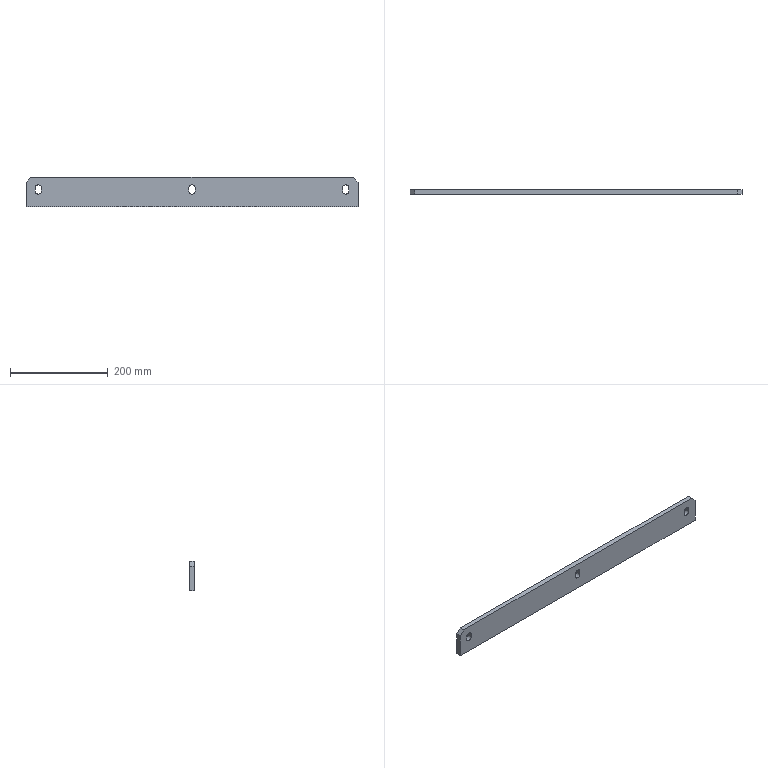Part | NX | features solid 2 | 1 solid | 20 faces | box 680 x 10 x 60 mm | volume 400678 mm3 | plane 14 | cylinder 6 | commonest cylinder face diameters 13 x6
STEP:
#1=CARTESIAN_POINT('',(-390.,10.,-530.));
#2=VERTEX_POINT('',#1);
#3=CARTESIAN_POINT('',(-380.,10.,-540.));
#4=VERTEX_POINT('',#3);
#5=CARTESIAN_POINT('',(-380.,10.,-540.));
#6=DIRECTION('',(0.7071,0.,-0.7071));
#7=VECTOR('',#6,1000.);
#8=LINE('',#5,#7);
#9=EDGE_CURVE('',#2,#4,#8,.T.);
#10=ORIENTED_EDGE('',*,*,#9,.F.);
#11=CARTESIAN_POINT('',(-390.,0.,-530.));
#12=VERTEX_POINT('',#11);
#13=CARTESIAN_POINT('',(-390.,0.,-530.));
#14=DIRECTION('',(0.,1.,0.));
#15=VECTOR('',#14,1000.);
#16=LINE('',#13,#15);
#17=EDGE_CURVE('',#12,#2,#16,.T.);
#18=ORIENTED_EDGE('',*,*,#17,.F.);
#19=CARTESIAN_POINT('',(-380.,0.,-540.));
#20=VERTEX_POINT('',#19);
#21=CARTESIAN_POINT('',(-655.,0.,-265.));
#22=DIRECTION('',(-0.7071,0.,0.7071));
#23=VECTOR('',#22,1000.);
#24=LINE('',#21,#23);
#25=EDGE_CURVE('',#20,#12,#24,.T.);
#26=ORIENTED_EDGE('',*,*,#25,.F.);
#27=CARTESIAN_POINT('',(-380.,10.,-540.));
#28=DIRECTION('',(0.,-1.,0.));
#29=VECTOR('',#28,1000.);
#30=LINE('',#27,#29);
#31=EDGE_CURVE('',#4,#20,#30,.T.);
#32=ORIENTED_EDGE('',*,*,#31,.F.);
#33=EDGE_LOOP('',(#10,#18,#26,#32));
#34=FACE_BOUND('',#33,.T.);
#35=CARTESIAN_POINT('',(-380.,10.,-540.));
#36=DIRECTION('',(-0.7071,0.,-0.7071));
#37=DIRECTION('',(-0.7071,0.,0.7071));
#38=AXIS2_PLACEMENT_3D('',#35,#36,#37);
#39=PLANE('',#38);
#40=ADVANCED_FACE('',(#34),#39,.F.);
#41=CARTESIAN_POINT('',(-1060.,10.,-540.));
#42=VERTEX_POINT('',#41);
#43=CARTESIAN_POINT('',(-1050.,10.,-530.));
#44=VERTEX_POINT('',#43);
#45=CARTESIAN_POINT('',(-1050.,10.,-530.));
#46=DIRECTION('',(0.7071,0.,0.7071));
#47=VECTOR('',#46,1000.);
#48=LINE('',#45,#47);
#49=EDGE_CURVE('',#42,#44,#48,.T.);
#50=ORIENTED_EDGE('',*,*,#49,.F.);
#51=CARTESIAN_POINT('',(-1060.,0.,-540.));
#52=VERTEX_POINT('',#51);
#53=CARTESIAN_POINT('',(-1060.,10.,-540.));
#54=DIRECTION('',(0.,1.,0.));
#55=VECTOR('',#54,1000.);
#56=LINE('',#53,#55);
#57=EDGE_CURVE('',#52,#42,#56,.T.);
#58=ORIENTED_EDGE('',*,*,#57,.F.);
#59=CARTESIAN_POINT('',(-1050.,0.,-530.));
#60=VERTEX_POINT('',#59);
#61=CARTESIAN_POINT('',(-1055.,0.,-535.));
#62=DIRECTION('',(-0.7071,0.,-0.7071));
#63=VECTOR('',#62,1000.);
#64=LINE('',#61,#63);
#65=EDGE_CURVE('',#60,#52,#64,.T.);
#66=ORIENTED_EDGE('',*,*,#65,.F.);
#67=CARTESIAN_POINT('',(-1050.,0.,-530.));
#68=DIRECTION('',(0.,-1.,0.));
#69=VECTOR('',#68,1000.);
#70=LINE('',#67,#69);
#71=EDGE_CURVE('',#44,#60,#70,.T.);
#72=ORIENTED_EDGE('',*,*,#71,.F.);
#73=EDGE_LOOP('',(#50,#58,#66,#72));
#74=FACE_BOUND('',#73,.T.);
#75=CARTESIAN_POINT('',(-1050.,0.,-530.));
#76=DIRECTION('',(0.7071,0.,-0.7071));
#77=DIRECTION('',(0.,-1.,0.));
#78=AXIS2_PLACEMENT_3D('',#75,#76,#77);
#79=PLANE('',#78);
#80=ADVANCED_FACE('',(#74),#79,.F.);
#81=CARTESIAN_POINT('',(-1028.5,0.,-558.001));
#82=VERTEX_POINT('',#81);
#83=CARTESIAN_POINT('',(-1028.5,0.,-552.001));
#84=VERTEX_POINT('',#83);
#85=CARTESIAN_POINT('',(-1028.5,0.,-600.));
#86=DIRECTION('',(0.,0.,1.));
#87=VECTOR('',#86,1000.);
#88=LINE('',#85,#87);
#89=EDGE_CURVE('',#82,#84,#88,.T.);
#90=ORIENTED_EDGE('',*,*,#89,.T.);
#91=CARTESIAN_POINT('',(-1028.5,10.,-552.001));
#92=VERTEX_POINT('',#91);
#93=CARTESIAN_POINT('',(-1028.5,-672.715,-552.001));
#94=DIRECTION('',(0.,1.,0.));
#95=VECTOR('',#94,1000.);
#96=LINE('',#93,#95);
#97=EDGE_CURVE('',#84,#92,#96,.T.);
#98=ORIENTED_EDGE('',*,*,#97,.T.);
#99=CARTESIAN_POINT('',(-1028.5,10.,-558.001));
#100=VERTEX_POINT('',#99);
#101=CARTESIAN_POINT('',(-1028.5,10.,-552.001));
#102=DIRECTION('',(0.,0.,-1.));
#103=VECTOR('',#102,1000.);
#104=LINE('',#101,#103);
#105=EDGE_CURVE('',#92,#100,#104,.T.);
#106=ORIENTED_EDGE('',*,*,#105,.T.);
#107=CARTESIAN_POINT('',(-1028.5,-672.715,-558.001));
#108=DIRECTION('',(0.,1.,0.));
#109=VECTOR('',#108,1000.);
#110=LINE('',#107,#109);
#111=EDGE_CURVE('',#82,#100,#110,.T.);
#112=ORIENTED_EDGE('',*,*,#111,.F.);
#113=EDGE_LOOP('',(#90,#98,#106,#112));
#114=FACE_BOUND('',#113,.T.);
#115=CARTESIAN_POINT('',(-1028.5,-672.715,-552.001));
#116=DIRECTION('',(1.,0.,0.));
#117=DIRECTION('',(0.,0.,-1.));
#118=AXIS2_PLACEMENT_3D('',#115,#116,#117);
#119=PLANE('',#118);
#120=ADVANCED_FACE('',(#114),#119,.F.);
#121=CARTESIAN_POINT('',(-1041.5,0.,-552.001));
#122=VERTEX_POINT('',#121);
#123=CARTESIAN_POINT('',(-1035.,0.,-552.001));
#124=DIRECTION('',(0.,-1.,0.));
#125=DIRECTION('',(1.,0.,0.));
#126=AXIS2_PLACEMENT_3D('',#123,#124,#125);
#127=CIRCLE('',#126,6.5);
#128=EDGE_CURVE('',#84,#122,#127,.T.);
#129=ORIENTED_EDGE('',*,*,#128,.T.);
#130=CARTESIAN_POINT('',(-1041.5,10.,-552.001));
#131=VERTEX_POINT('',#130);
#132=CARTESIAN_POINT('',(-1041.5,-672.715,-552.001));
#133=DIRECTION('',(0.,1.,0.));
#134=VECTOR('',#133,1000.);
#135=LINE('',#132,#134);
#136=EDGE_CURVE('',#122,#131,#135,.T.);
#137=ORIENTED_EDGE('',*,*,#136,.T.);
#138=CARTESIAN_POINT('',(-1035.,10.,-552.001));
#139=DIRECTION('',(0.,1.,0.));
#140=DIRECTION('',(-1.,0.,0.));
#141=AXIS2_PLACEMENT_3D('',#138,#139,#140);
#142=CIRCLE('',#141,6.5);
#143=EDGE_CURVE('',#131,#92,#142,.T.);
#144=ORIENTED_EDGE('',*,*,#143,.T.);
#145=ORIENTED_EDGE('',*,*,#97,.F.);
#146=EDGE_LOOP('',(#129,#137,#144,#145));
#147=FACE_BOUND('',#146,.T.);
#148=CARTESIAN_POINT('',(-1035.,-672.715,-552.001));
#149=DIRECTION('',(0.,1.,0.));
#150=DIRECTION('',(-1.,0.,0.));
#151=AXIS2_PLACEMENT_3D('',#148,#149,#150);
#152=CYLINDRICAL_SURFACE('',#151,6.5);
#153=ADVANCED_FACE('',(#147),#152,.F.);
#154=CARTESIAN_POINT('',(-1041.5,0.,-558.001));
#155=VERTEX_POINT('',#154);
#156=CARTESIAN_POINT('',(-1041.5,0.,-600.));
#157=DIRECTION('',(0.,0.,-1.));
#158=VECTOR('',#157,1000.);
#159=LINE('',#156,#158);
#160=EDGE_CURVE('',#122,#155,#159,.T.);
#161=ORIENTED_EDGE('',*,*,#160,.T.);
#162=CARTESIAN_POINT('',(-1041.5,10.,-558.001));
#163=VERTEX_POINT('',#162);
#164=CARTESIAN_POINT('',(-1041.5,-672.715,-558.001));
#165=DIRECTION('',(0.,1.,0.));
#166=VECTOR('',#165,1000.);
#167=LINE('',#164,#166);
#168=EDGE_CURVE('',#155,#163,#167,.T.);
#169=ORIENTED_EDGE('',*,*,#168,.T.);
#170=CARTESIAN_POINT('',(-1041.5,10.,-552.001));
#171=DIRECTION('',(0.,0.,1.));
#172=VECTOR('',#171,1000.);
#173=LINE('',#170,#172);
#174=EDGE_CURVE('',#163,#131,#173,.T.);
#175=ORIENTED_EDGE('',*,*,#174,.T.);
#176=ORIENTED_EDGE('',*,*,#136,.F.);
#177=EDGE_LOOP('',(#161,#169,#175,#176));
#178=FACE_BOUND('',#177,.T.);
#179=CARTESIAN_POINT('',(-1041.5,-672.715,-552.001));
#180=DIRECTION('',(-1.,0.,0.));
#181=DIRECTION('',(0.,1.,0.));
#182=AXIS2_PLACEMENT_3D('',#179,#180,#181);
#183=PLANE('',#182);
#184=ADVANCED_FACE('',(#178),#183,.F.);
#185=CARTESIAN_POINT('',(-1035.,0.,-558.001));
#186=DIRECTION('',(0.,-1.,0.));
#187=DIRECTION('',(1.,0.,0.));
#188=AXIS2_PLACEMENT_3D('',#185,#186,#187);
#189=CIRCLE('',#188,6.5);
#190=EDGE_CURVE('',#155,#82,#189,.T.);
#191=ORIENTED_EDGE('',*,*,#190,.T.);
#192=ORIENTED_EDGE('',*,*,#111,.T.);
#193=CARTESIAN_POINT('',(-1035.,10.,-558.001));
#194=DIRECTION('',(0.,1.,0.));
#195=DIRECTION('',(1.,0.,0.));
#196=AXIS2_PLACEMENT_3D('',#193,#194,#195);
#197=CIRCLE('',#196,6.5);
#198=EDGE_CURVE('',#100,#163,#197,.T.);
#199=ORIENTED_EDGE('',*,*,#198,.T.);
#200=ORIENTED_EDGE('',*,*,#168,.F.);
#201=EDGE_LOOP('',(#191,#192,#199,#200));
#202=FACE_BOUND('',#201,.T.);
#203=CARTESIAN_POINT('',(-1035.,-672.715,-558.001));
#204=DIRECTION('',(0.,1.,0.));
#205=DIRECTION('',(-1.,0.,0.));
#206=AXIS2_PLACEMENT_3D('',#203,#204,#205);
#207=CYLINDRICAL_SURFACE('',#206,6.5);
#208=ADVANCED_FACE('',(#202),#207,.F.);
#209=CARTESIAN_POINT('',(-713.5,0.,-558.001));
#210=VERTEX_POINT('',#209);
#211=CARTESIAN_POINT('',(-713.5,0.,-552.001));
#212=VERTEX_POINT('',#211);
#213=CARTESIAN_POINT('',(-713.5,0.,-600.));
#214=DIRECTION('',(0.,0.,1.));
#215=VECTOR('',#214,1000.);
#216=LINE('',#213,#215);
#217=EDGE_CURVE('',#210,#212,#216,.T.);
#218=ORIENTED_EDGE('',*,*,#217,.T.);
#219=CARTESIAN_POINT('',(-713.5,10.,-552.001));
#220=VERTEX_POINT('',#219);
#221=CARTESIAN_POINT('',(-713.5,-672.715,-552.001));
#222=DIRECTION('',(0.,1.,0.));
#223=VECTOR('',#222,1000.);
#224=LINE('',#221,#223);
#225=EDGE_CURVE('',#212,#220,#224,.T.);
#226=ORIENTED_EDGE('',*,*,#225,.T.);
#227=CARTESIAN_POINT('',(-713.5,10.,-558.001));
#228=VERTEX_POINT('',#227);
#229=CARTESIAN_POINT('',(-713.5,10.,-552.001));
#230=DIRECTION('',(0.,0.,-1.));
#231=VECTOR('',#230,1000.);
#232=LINE('',#229,#231);
#233=EDGE_CURVE('',#220,#228,#232,.T.);
#234=ORIENTED_EDGE('',*,*,#233,.T.);
#235=CARTESIAN_POINT('',(-713.5,-672.715,-558.001));
#236=DIRECTION('',(0.,1.,0.));
#237=VECTOR('',#236,1000.);
#238=LINE('',#235,#237);
#239=EDGE_CURVE('',#210,#228,#238,.T.);
#240=ORIENTED_EDGE('',*,*,#239,.F.);
#241=EDGE_LOOP('',(#218,#226,#234,#240));
#242=FACE_BOUND('',#241,.T.);
#243=CARTESIAN_POINT('',(-713.5,-672.715,-552.001));
#244=DIRECTION('',(1.,0.,0.));
#245=DIRECTION('',(0.,0.,-1.));
#246=AXIS2_PLACEMENT_3D('',#243,#244,#245);
#247=PLANE('',#246);
#248=ADVANCED_FACE('',(#242),#247,.F.);
#249=CARTESIAN_POINT('',(-726.5,0.,-552.001));
#250=VERTEX_POINT('',#249);
#251=CARTESIAN_POINT('',(-720.,0.,-552.001));
#252=DIRECTION('',(0.,-1.,0.));
#253=DIRECTION('',(1.,0.,0.));
#254=AXIS2_PLACEMENT_3D('',#251,#252,#253);
#255=CIRCLE('',#254,6.5);
#256=EDGE_CURVE('',#212,#250,#255,.T.);
#257=ORIENTED_EDGE('',*,*,#256,.T.);
#258=CARTESIAN_POINT('',(-726.5,10.,-552.001));
#259=VERTEX_POINT('',#258);
#260=CARTESIAN_POINT('',(-726.5,-672.715,-552.001));
#261=DIRECTION('',(0.,1.,0.));
#262=VECTOR('',#261,1000.);
#263=LINE('',#260,#262);
#264=EDGE_CURVE('',#250,#259,#263,.T.);
#265=ORIENTED_EDGE('',*,*,#264,.T.);
#266=CARTESIAN_POINT('',(-720.,10.,-552.001));
#267=DIRECTION('',(0.,1.,0.));
#268=DIRECTION('',(-1.,0.,0.));
#269=AXIS2_PLACEMENT_3D('',#266,#267,#268);
#270=CIRCLE('',#269,6.5);
#271=EDGE_CURVE('',#259,#220,#270,.T.);
#272=ORIENTED_EDGE('',*,*,#271,.T.);
#273=ORIENTED_EDGE('',*,*,#225,.F.);
#274=EDGE_LOOP('',(#257,#265,#272,#273));
#275=FACE_BOUND('',#274,.T.);
#276=CARTESIAN_POINT('',(-720.,-672.715,-552.001));
#277=DIRECTION('',(0.,1.,0.));
#278=DIRECTION('',(-1.,0.,0.));
#279=AXIS2_PLACEMENT_3D('',#276,#277,#278);
#280=CYLINDRICAL_SURFACE('',#279,6.5);
#281=ADVANCED_FACE('',(#275),#280,.F.);
#282=CARTESIAN_POINT('',(-726.5,0.,-558.001));
#283=VERTEX_POINT('',#282);
#284=CARTESIAN_POINT('',(-726.5,0.,-600.));
#285=DIRECTION('',(0.,0.,-1.));
#286=VECTOR('',#285,1000.);
#287=LINE('',#284,#286);
#288=EDGE_CURVE('',#250,#283,#287,.T.);
#289=ORIENTED_EDGE('',*,*,#288,.T.);
#290=CARTESIAN_POINT('',(-726.5,10.,-558.001));
#291=VERTEX_POINT('',#290);
#292=CARTESIAN_POINT('',(-726.5,-672.715,-558.001));
#293=DIRECTION('',(0.,1.,0.));
#294=VECTOR('',#293,1000.);
#295=LINE('',#292,#294);
#296=EDGE_CURVE('',#283,#291,#295,.T.);
#297=ORIENTED_EDGE('',*,*,#296,.T.);
#298=CARTESIAN_POINT('',(-726.5,10.,-552.001));
#299=DIRECTION('',(0.,0.,1.));
#300=VECTOR('',#299,1000.);
#301=LINE('',#298,#300);
#302=EDGE_CURVE('',#291,#259,#301,.T.);
#303=ORIENTED_EDGE('',*,*,#302,.T.);
#304=ORIENTED_EDGE('',*,*,#264,.F.);
#305=EDGE_LOOP('',(#289,#297,#303,#304));
#306=FACE_BOUND('',#305,.T.);
#307=CARTESIAN_POINT('',(-726.5,-672.715,-552.001));
#308=DIRECTION('',(-1.,0.,0.));
#309=DIRECTION('',(0.,1.,0.));
#310=AXIS2_PLACEMENT_3D('',#307,#308,#309);
#311=PLANE('',#310);
#312=ADVANCED_FACE('',(#306),#311,.F.);
#313=CARTESIAN_POINT('',(-720.,0.,-558.001));
#314=DIRECTION('',(0.,-1.,0.));
#315=DIRECTION('',(1.,0.,0.));
#316=AXIS2_PLACEMENT_3D('',#313,#314,#315);
#317=CIRCLE('',#316,6.5);
#318=EDGE_CURVE('',#283,#210,#317,.T.);
#319=ORIENTED_EDGE('',*,*,#318,.T.);
#320=ORIENTED_EDGE('',*,*,#239,.T.);
#321=CARTESIAN_POINT('',(-720.,10.,-558.001));
#322=DIRECTION('',(0.,1.,0.));
#323=DIRECTION('',(1.,0.,0.));
#324=AXIS2_PLACEMENT_3D('',#321,#322,#323);
#325=CIRCLE('',#324,6.5);
#326=EDGE_CURVE('',#228,#291,#325,.T.);
#327=ORIENTED_EDGE('',*,*,#326,.T.);
#328=ORIENTED_EDGE('',*,*,#296,.F.);
#329=EDGE_LOOP('',(#319,#320,#327,#328));
#330=FACE_BOUND('',#329,.T.);
#331=CARTESIAN_POINT('',(-720.,-672.715,-558.001));
#332=DIRECTION('',(0.,1.,0.));
#333=DIRECTION('',(-1.,0.,0.));
#334=AXIS2_PLACEMENT_3D('',#331,#332,#333);
#335=CYLINDRICAL_SURFACE('',#334,6.5);
#336=ADVANCED_FACE('',(#330),#335,.F.);
#337=CARTESIAN_POINT('',(-398.5,0.,-558.001));
#338=VERTEX_POINT('',#337);
#339=CARTESIAN_POINT('',(-398.5,0.,-552.001));
#340=VERTEX_POINT('',#339);
#341=CARTESIAN_POINT('',(-398.5,0.,-600.));
#342=DIRECTION('',(0.,0.,1.));
#343=VECTOR('',#342,1000.);
#344=LINE('',#341,#343);
#345=EDGE_CURVE('',#338,#340,#344,.T.);
#346=ORIENTED_EDGE('',*,*,#345,.T.);
#347=CARTESIAN_POINT('',(-398.5,10.,-552.001));
#348=VERTEX_POINT('',#347);
#349=CARTESIAN_POINT('',(-398.5,-672.715,-552.001));
#350=DIRECTION('',(0.,1.,0.));
#351=VECTOR('',#350,1000.);
#352=LINE('',#349,#351);
#353=EDGE_CURVE('',#340,#348,#352,.T.);
#354=ORIENTED_EDGE('',*,*,#353,.T.);
#355=CARTESIAN_POINT('',(-398.5,10.,-558.001));
#356=VERTEX_POINT('',#355);
#357=CARTESIAN_POINT('',(-398.5,10.,-552.001));
#358=DIRECTION('',(0.,0.,-1.));
#359=VECTOR('',#358,1000.);
#360=LINE('',#357,#359);
#361=EDGE_CURVE('',#348,#356,#360,.T.);
#362=ORIENTED_EDGE('',*,*,#361,.T.);
#363=CARTESIAN_POINT('',(-398.5,-672.715,-558.001));
#364=DIRECTION('',(0.,1.,0.));
#365=VECTOR('',#364,1000.);
#366=LINE('',#363,#365);
#367=EDGE_CURVE('',#338,#356,#366,.T.);
#368=ORIENTED_EDGE('',*,*,#367,.F.);
#369=EDGE_LOOP('',(#346,#354,#362,#368));
#370=FACE_BOUND('',#369,.T.);
#371=CARTESIAN_POINT('',(-398.5,-672.715,-552.001));
#372=DIRECTION('',(1.,0.,0.));
#373=DIRECTION('',(0.,0.,-1.));
#374=AXIS2_PLACEMENT_3D('',#371,#372,#373);
#375=PLANE('',#374);
#376=ADVANCED_FACE('',(#370),#375,.F.);
#377=CARTESIAN_POINT('',(-411.5,0.,-552.001));
#378=VERTEX_POINT('',#377);
#379=CARTESIAN_POINT('',(-405.,0.,-552.001));
#380=DIRECTION('',(0.,-1.,0.));
#381=DIRECTION('',(1.,0.,0.));
#382=AXIS2_PLACEMENT_3D('',#379,#380,#381);
#383=CIRCLE('',#382,6.5);
#384=EDGE_CURVE('',#340,#378,#383,.T.);
#385=ORIENTED_EDGE('',*,*,#384,.T.);
#386=CARTESIAN_POINT('',(-411.5,10.,-552.001));
#387=VERTEX_POINT('',#386);
#388=CARTESIAN_POINT('',(-411.5,-672.715,-552.001));
#389=DIRECTION('',(0.,1.,0.));
#390=VECTOR('',#389,1000.);
#391=LINE('',#388,#390);
#392=EDGE_CURVE('',#378,#387,#391,.T.);
#393=ORIENTED_EDGE('',*,*,#392,.T.);
#394=CARTESIAN_POINT('',(-405.,10.,-552.001));
#395=DIRECTION('',(0.,1.,0.));
#396=DIRECTION('',(-1.,0.,0.));
#397=AXIS2_PLACEMENT_3D('',#394,#395,#396);
#398=CIRCLE('',#397,6.5);
#399=EDGE_CURVE('',#387,#348,#398,.T.);
#400=ORIENTED_EDGE('',*,*,#399,.T.);
#401=ORIENTED_EDGE('',*,*,#353,.F.);
#402=EDGE_LOOP('',(#385,#393,#400,#401));
#403=FACE_BOUND('',#402,.T.);
#404=CARTESIAN_POINT('',(-405.,-672.715,-552.001));
#405=DIRECTION('',(0.,1.,0.));
#406=DIRECTION('',(-1.,0.,0.));
#407=AXIS2_PLACEMENT_3D('',#404,#405,#406);
#408=CYLINDRICAL_SURFACE('',#407,6.5);
#409=ADVANCED_FACE('',(#403),#408,.F.);
#410=CARTESIAN_POINT('',(-411.5,0.,-558.001));
#411=VERTEX_POINT('',#410);
#412=CARTESIAN_POINT('',(-411.5,0.,-600.));
#413=DIRECTION('',(0.,0.,-1.));
#414=VECTOR('',#413,1000.);
#415=LINE('',#412,#414);
#416=EDGE_CURVE('',#378,#411,#415,.T.);
#417=ORIENTED_EDGE('',*,*,#416,.T.);
#418=CARTESIAN_POINT('',(-411.5,10.,-558.001));
#419=VERTEX_POINT('',#418);
#420=CARTESIAN_POINT('',(-411.5,-672.715,-558.001));
#421=DIRECTION('',(0.,1.,0.));
#422=VECTOR('',#421,1000.);
#423=LINE('',#420,#422);
#424=EDGE_CURVE('',#411,#419,#423,.T.);
#425=ORIENTED_EDGE('',*,*,#424,.T.);
#426=CARTESIAN_POINT('',(-411.5,10.,-552.001));
#427=DIRECTION('',(0.,0.,1.));
#428=VECTOR('',#427,1000.);
#429=LINE('',#426,#428);
#430=EDGE_CURVE('',#419,#387,#429,.T.);
#431=ORIENTED_EDGE('',*,*,#430,.T.);
#432=ORIENTED_EDGE('',*,*,#392,.F.);
#433=EDGE_LOOP('',(#417,#425,#431,#432));
#434=FACE_BOUND('',#433,.T.);
#435=CARTESIAN_POINT('',(-411.5,-672.715,-552.001));
#436=DIRECTION('',(-1.,0.,0.));
#437=DIRECTION('',(0.,1.,0.));
#438=AXIS2_PLACEMENT_3D('',#435,#436,#437);
#439=PLANE('',#438);
#440=ADVANCED_FACE('',(#434),#439,.F.);
#441=CARTESIAN_POINT('',(-405.,0.,-558.001));
#442=DIRECTION('',(0.,-1.,0.));
#443=DIRECTION('',(1.,0.,0.));
#444=AXIS2_PLACEMENT_3D('',#441,#442,#443);
#445=CIRCLE('',#444,6.5);
#446=EDGE_CURVE('',#411,#338,#445,.T.);
#447=ORIENTED_EDGE('',*,*,#446,.T.);
#448=ORIENTED_EDGE('',*,*,#367,.T.);
#449=CARTESIAN_POINT('',(-405.,10.,-558.001));
#450=DIRECTION('',(0.,1.,0.));
#451=DIRECTION('',(1.,0.,0.));
#452=AXIS2_PLACEMENT_3D('',#449,#450,#451);
#453=CIRCLE('',#452,6.5);
#454=EDGE_CURVE('',#356,#419,#453,.T.);
#455=ORIENTED_EDGE('',*,*,#454,.T.);
#456=ORIENTED_EDGE('',*,*,#424,.F.);
#457=EDGE_LOOP('',(#447,#448,#455,#456));
#458=FACE_BOUND('',#457,.T.);
#459=CARTESIAN_POINT('',(-405.,-672.715,-558.001));
#460=DIRECTION('',(0.,1.,0.));
#461=DIRECTION('',(-1.,0.,0.));
#462=AXIS2_PLACEMENT_3D('',#459,#460,#461);
#463=CYLINDRICAL_SURFACE('',#462,6.5);
#464=ADVANCED_FACE('',(#458),#463,.F.);
#465=CARTESIAN_POINT('',(-380.,10.,-590.));
#466=VERTEX_POINT('',#465);
#467=CARTESIAN_POINT('',(-380.,10.,-600.));
#468=DIRECTION('',(0.,0.,1.));
#469=VECTOR('',#468,1000.);
#470=LINE('',#467,#469);
#471=EDGE_CURVE('',#466,#4,#470,.T.);
#472=ORIENTED_EDGE('',*,*,#471,.T.);
#473=ORIENTED_EDGE('',*,*,#31,.T.);
#474=CARTESIAN_POINT('',(-380.,0.,-590.));
#475=VERTEX_POINT('',#474);
#476=CARTESIAN_POINT('',(-380.,0.,-600.));
#477=DIRECTION('',(0.,0.,1.));
#478=VECTOR('',#477,1000.);
#479=LINE('',#476,#478);
#480=EDGE_CURVE('',#475,#20,#479,.T.);
#481=ORIENTED_EDGE('',*,*,#480,.F.);
#482=CARTESIAN_POINT('',(-380.,10.,-590.));
#483=DIRECTION('',(0.,1.,0.));
#484=VECTOR('',#483,1000.);
#485=LINE('',#482,#484);
#486=EDGE_CURVE('',#475,#466,#485,.T.);
#487=ORIENTED_EDGE('',*,*,#486,.T.);
#488=EDGE_LOOP('',(#472,#473,#481,#487));
#489=FACE_BOUND('',#488,.T.);
#490=CARTESIAN_POINT('',(-380.,10.,-600.));
#491=DIRECTION('',(-1.,0.,0.));
#492=DIRECTION('',(0.,1.,0.));
#493=AXIS2_PLACEMENT_3D('',#490,#491,#492);
#494=PLANE('',#493);
#495=ADVANCED_FACE('',(#489),#494,.F.);
#496=CARTESIAN_POINT('',(-990.,10.,-530.));
#497=DIRECTION('',(-1.,0.,0.));
#498=VECTOR('',#497,1000.);
#499=LINE('',#496,#498);
#500=EDGE_CURVE('',#2,#44,#499,.T.);
#501=ORIENTED_EDGE('',*,*,#500,.T.);
#502=ORIENTED_EDGE('',*,*,#71,.T.);
#503=CARTESIAN_POINT('',(-990.,0.,-530.));
#504=DIRECTION('',(-1.,0.,0.));
#505=VECTOR('',#504,1000.);
#506=LINE('',#503,#505);
#507=EDGE_CURVE('',#12,#60,#506,.T.);
#508=ORIENTED_EDGE('',*,*,#507,.F.);
#509=ORIENTED_EDGE('',*,*,#17,.T.);
#510=EDGE_LOOP('',(#501,#502,#508,#509));
#511=FACE_BOUND('',#510,.T.);
#512=CARTESIAN_POINT('',(-990.,0.,-530.));
#513=DIRECTION('',(0.,0.,-1.));
#514=DIRECTION('',(-1.,0.,0.));
#515=AXIS2_PLACEMENT_3D('',#512,#513,#514);
#516=PLANE('',#515);
#517=ADVANCED_FACE('',(#511),#516,.F.);
#518=ORIENTED_EDGE('',*,*,#446,.F.);
#519=ORIENTED_EDGE('',*,*,#416,.F.);
#520=ORIENTED_EDGE('',*,*,#384,.F.);
#521=ORIENTED_EDGE('',*,*,#345,.F.);
#522=EDGE_LOOP('',(#518,#519,#520,#521));
#523=FACE_BOUND('',#522,.T.);
#524=ORIENTED_EDGE('',*,*,#318,.F.);
#525=ORIENTED_EDGE('',*,*,#288,.F.);
#526=ORIENTED_EDGE('',*,*,#256,.F.);
#527=ORIENTED_EDGE('',*,*,#217,.F.);
#528=EDGE_LOOP('',(#524,#525,#526,#527));
#529=FACE_BOUND('',#528,.T.);
#530=ORIENTED_EDGE('',*,*,#190,.F.);
#531=ORIENTED_EDGE('',*,*,#160,.F.);
#532=ORIENTED_EDGE('',*,*,#128,.F.);
#533=ORIENTED_EDGE('',*,*,#89,.F.);
#534=EDGE_LOOP('',(#530,#531,#532,#533));
#535=FACE_BOUND('',#534,.T.);
#536=ORIENTED_EDGE('',*,*,#507,.T.);
#537=ORIENTED_EDGE('',*,*,#65,.T.);
#538=CARTESIAN_POINT('',(-1060.,0.,-590.));
#539=VERTEX_POINT('',#538);
#540=CARTESIAN_POINT('',(-1060.,0.,-600.));
#541=DIRECTION('',(0.,0.,-1.));
#542=VECTOR('',#541,1000.);
#543=LINE('',#540,#542);
#544=EDGE_CURVE('',#52,#539,#543,.T.);
#545=ORIENTED_EDGE('',*,*,#544,.T.);
#546=CARTESIAN_POINT('',(-490.,0.,-590.));
#547=DIRECTION('',(1.,0.,0.));
#548=VECTOR('',#547,1000.);
#549=LINE('',#546,#548);
#550=EDGE_CURVE('',#539,#475,#549,.T.);
#551=ORIENTED_EDGE('',*,*,#550,.T.);
#552=ORIENTED_EDGE('',*,*,#480,.T.);
#553=ORIENTED_EDGE('',*,*,#25,.T.);
#554=EDGE_LOOP('',(#536,#537,#545,#551,#552,#553));
#555=FACE_BOUND('',#554,.T.);
#556=CARTESIAN_POINT('',(-990.,0.,-600.));
#557=DIRECTION('',(0.,-1.,0.));
#558=DIRECTION('',(-1.,0.,0.));
#559=AXIS2_PLACEMENT_3D('',#556,#557,#558);
#560=PLANE('',#559);
#561=ADVANCED_FACE('',(#523,#529,#535,#555),#560,.T.);
#562=ORIENTED_EDGE('',*,*,#486,.F.);
#563=ORIENTED_EDGE('',*,*,#550,.F.);
#564=CARTESIAN_POINT('',(-1060.,10.,-590.));
#565=VERTEX_POINT('',#564);
#566=CARTESIAN_POINT('',(-1060.,10.,-590.));
#567=DIRECTION('',(0.,1.,0.));
#568=VECTOR('',#567,1000.);
#569=LINE('',#566,#568);
#570=EDGE_CURVE('',#539,#565,#569,.T.);
#571=ORIENTED_EDGE('',*,*,#570,.T.);
#572=CARTESIAN_POINT('',(-490.,10.,-590.));
#573=DIRECTION('',(1.,0.,0.));
#574=VECTOR('',#573,1000.);
#575=LINE('',#572,#574);
#576=EDGE_CURVE('',#565,#466,#575,.T.);
#577=ORIENTED_EDGE('',*,*,#576,.T.);
#578=EDGE_LOOP('',(#562,#563,#571,#577));
#579=FACE_BOUND('',#578,.T.);
#580=CARTESIAN_POINT('',(-490.,10.,-590.));
#581=DIRECTION('',(0.,0.,1.));
#582=DIRECTION('',(0.,-1.,0.));
#583=AXIS2_PLACEMENT_3D('',#580,#581,#582);
#584=PLANE('',#583);
#585=ADVANCED_FACE('',(#579),#584,.F.);
#586=ORIENTED_EDGE('',*,*,#430,.F.);
#587=ORIENTED_EDGE('',*,*,#454,.F.);
#588=ORIENTED_EDGE('',*,*,#361,.F.);
#589=ORIENTED_EDGE('',*,*,#399,.F.);
#590=EDGE_LOOP('',(#586,#587,#588,#589));
#591=FACE_BOUND('',#590,.T.);
#592=ORIENTED_EDGE('',*,*,#302,.F.);
#593=ORIENTED_EDGE('',*,*,#326,.F.);
#594=ORIENTED_EDGE('',*,*,#233,.F.);
#595=ORIENTED_EDGE('',*,*,#271,.F.);
#596=EDGE_LOOP('',(#592,#593,#594,#595));
#597=FACE_BOUND('',#596,.T.);
#598=ORIENTED_EDGE('',*,*,#174,.F.);
#599=ORIENTED_EDGE('',*,*,#198,.F.);
#600=ORIENTED_EDGE('',*,*,#105,.F.);
#601=ORIENTED_EDGE('',*,*,#143,.F.);
#602=EDGE_LOOP('',(#598,#599,#600,#601));
#603=FACE_BOUND('',#602,.T.);
#604=CARTESIAN_POINT('',(-1060.,10.,-600.));
#605=DIRECTION('',(0.,0.,1.));
#606=VECTOR('',#605,1000.);
#607=LINE('',#604,#606);
#608=EDGE_CURVE('',#565,#42,#607,.T.);
#609=ORIENTED_EDGE('',*,*,#608,.T.);
#610=ORIENTED_EDGE('',*,*,#49,.T.);
#611=ORIENTED_EDGE('',*,*,#500,.F.);
#612=ORIENTED_EDGE('',*,*,#9,.T.);
#613=ORIENTED_EDGE('',*,*,#471,.F.);
#614=ORIENTED_EDGE('',*,*,#576,.F.);
#615=EDGE_LOOP('',(#609,#610,#611,#612,#613,#614));
#616=FACE_BOUND('',#615,.T.);
#617=CARTESIAN_POINT('',(-990.,10.,-600.));
#618=DIRECTION('',(0.,-1.,0.));
#619=DIRECTION('',(-1.,0.,0.));
#620=AXIS2_PLACEMENT_3D('',#617,#618,#619);
#621=PLANE('',#620);
#622=ADVANCED_FACE('',(#591,#597,#603,#616),#621,.F.);
#623=ORIENTED_EDGE('',*,*,#544,.F.);
#624=ORIENTED_EDGE('',*,*,#57,.T.);
#625=ORIENTED_EDGE('',*,*,#608,.F.);
#626=ORIENTED_EDGE('',*,*,#570,.F.);
#627=EDGE_LOOP('',(#623,#624,#625,#626));
#628=FACE_BOUND('',#627,.T.);
#629=CARTESIAN_POINT('',(-1060.,10.,-600.));
#630=DIRECTION('',(1.,0.,0.));
#631=DIRECTION('',(0.,0.,-1.));
#632=AXIS2_PLACEMENT_3D('',#629,#630,#631);
#633=PLANE('',#632);
#634=ADVANCED_FACE('',(#628),#633,.F.);
#635=CLOSED_SHELL('',(#40,#80,#120,#153,#184,#208,#248,#281,#312,#336,#376,#409,#440,#464,#495,#517,#561,#585,#622,#634));
#636=MANIFOLD_SOLID_BREP('',#635);
#637=(LENGTH_UNIT()NAMED_UNIT(*)SI_UNIT(.MILLI.,.METRE.));
#638=UNCERTAINTY_MEASURE_WITH_UNIT(LENGTH_MEASURE(0.00001),#637,'','');
#639=(NAMED_UNIT(*)PLANE_ANGLE_UNIT()SI_UNIT($,.RADIAN.));
#640=(NAMED_UNIT(*)SI_UNIT($,.STERADIAN.)SOLID_ANGLE_UNIT());
#641=(GEOMETRIC_REPRESENTATION_CONTEXT(3)GLOBAL_UNCERTAINTY_ASSIGNED_CONTEXT((#638))GLOBAL_UNIT_ASSIGNED_CONTEXT((#637,#639,#640))REPRESENTATION_CONTEXT('',''));
#642=ADVANCED_BREP_SHAPE_REPRESENTATION('',(#636),#641);